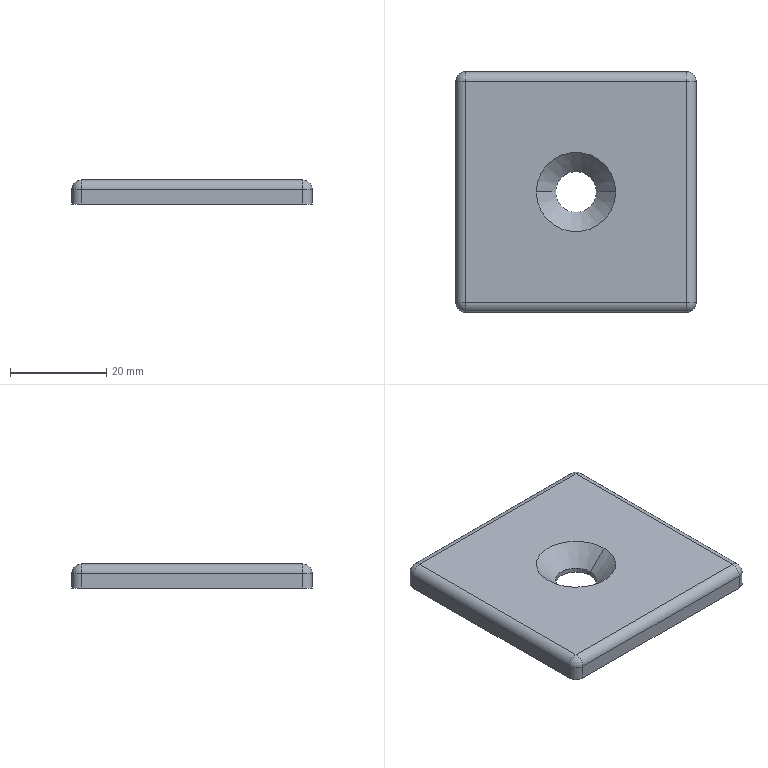Part | NX | features BREP 1 | 1 solid | 22 faces | box 50 x 50 x 5 mm | volume 11752 mm3 | cylinder 10 | plane 6 | sphere 4 | cone 2 | commonest cylinder face diameters 4 x8 8.5 x2
STEP:
#1=CARTESIAN_POINT('',(-4.25,0.,1.));
#2=VERTEX_POINT('',#1);
#3=CARTESIAN_POINT('',(4.25,0.,1.));
#4=VERTEX_POINT('',#3);
#5=CARTESIAN_POINT('',(0.,0.,1.));
#6=DIRECTION('',(0.,0.,1.));
#7=DIRECTION('',(-1.,0.,0.));
#8=AXIS2_PLACEMENT_3D('',#5,#6,#7);
#9=CIRCLE('',#8,4.25);
#10=EDGE_CURVE('',#2,#4,#9,.T.);
#11=ORIENTED_EDGE('',*,*,#10,.F.);
#12=CARTESIAN_POINT('',(-8.25,0.,5.));
#13=VERTEX_POINT('',#12);
#14=CARTESIAN_POINT('',(-4.25,0.,1.));
#15=DIRECTION('',(-0.7071,0.,0.7071));
#16=VECTOR('',#15,1000.);
#17=LINE('',#14,#16);
#18=EDGE_CURVE('',#13,#2,#17,.F.);
#19=ORIENTED_EDGE('',*,*,#18,.F.);
#20=CARTESIAN_POINT('',(8.25,0.,5.));
#21=VERTEX_POINT('',#20);
#22=CARTESIAN_POINT('',(0.,0.,5.));
#23=DIRECTION('',(0.,0.,-1.));
#24=DIRECTION('',(-1.,0.,0.));
#25=AXIS2_PLACEMENT_3D('',#22,#23,#24);
#26=CIRCLE('',#25,8.25);
#27=EDGE_CURVE('',#21,#13,#26,.T.);
#28=ORIENTED_EDGE('',*,*,#27,.F.);
#29=CARTESIAN_POINT('',(4.25,0.,1.));
#30=DIRECTION('',(0.7071,0.,0.7071));
#31=VECTOR('',#30,1000.);
#32=LINE('',#29,#31);
#33=EDGE_CURVE('',#21,#4,#32,.F.);
#34=ORIENTED_EDGE('',*,*,#33,.T.);
#35=EDGE_LOOP('',(#11,#19,#28,#34));
#36=FACE_BOUND('',#35,.T.);
#37=CARTESIAN_POINT('',(0.,0.,1.));
#38=DIRECTION('',(0.,0.,1.));
#39=DIRECTION('',(1.,0.,0.));
#40=AXIS2_PLACEMENT_3D('',#37,#38,#39);
#41=CONICAL_SURFACE('',#40,4.25,0.7854);
#42=ADVANCED_FACE('',(#36),#41,.F.);
#43=CARTESIAN_POINT('',(-4.25,0.,0.));
#44=VERTEX_POINT('',#43);
#45=CARTESIAN_POINT('',(4.25,0.,0.));
#46=VERTEX_POINT('',#45);
#47=CARTESIAN_POINT('',(0.,0.,0.));
#48=DIRECTION('',(0.,0.,1.));
#49=DIRECTION('',(1.,0.,0.));
#50=AXIS2_PLACEMENT_3D('',#47,#48,#49);
#51=CIRCLE('',#50,4.25);
#52=EDGE_CURVE('',#44,#46,#51,.T.);
#53=ORIENTED_EDGE('',*,*,#52,.F.);
#54=CARTESIAN_POINT('',(-4.25,0.,0.));
#55=DIRECTION('',(0.,0.,1.));
#56=VECTOR('',#55,1000.);
#57=LINE('',#54,#56);
#58=EDGE_CURVE('',#2,#44,#57,.F.);
#59=ORIENTED_EDGE('',*,*,#58,.F.);
#60=ORIENTED_EDGE('',*,*,#10,.T.);
#61=CARTESIAN_POINT('',(4.25,0.,0.));
#62=DIRECTION('',(0.,0.,1.));
#63=VECTOR('',#62,1000.);
#64=LINE('',#61,#63);
#65=EDGE_CURVE('',#4,#46,#64,.F.);
#66=ORIENTED_EDGE('',*,*,#65,.T.);
#67=EDGE_LOOP('',(#53,#59,#60,#66));
#68=FACE_BOUND('',#67,.T.);
#69=CARTESIAN_POINT('',(0.,0.,0.));
#70=DIRECTION('',(0.,0.,1.));
#71=DIRECTION('',(1.,0.,0.));
#72=AXIS2_PLACEMENT_3D('',#69,#70,#71);
#73=CYLINDRICAL_SURFACE('',#72,4.25);
#74=ADVANCED_FACE('',(#68),#73,.F.);
#75=CARTESIAN_POINT('',(25.,-23.,0.));
#76=VERTEX_POINT('',#75);
#77=CARTESIAN_POINT('',(25.,23.,0.));
#78=VERTEX_POINT('',#77);
#79=CARTESIAN_POINT('',(25.,-25.,0.));
#80=DIRECTION('',(0.,1.,0.));
#81=VECTOR('',#80,1000.);
#82=LINE('',#79,#81);
#83=EDGE_CURVE('',#76,#78,#82,.T.);
#84=ORIENTED_EDGE('',*,*,#83,.T.);
#85=CARTESIAN_POINT('',(25.,23.,3.));
#86=VERTEX_POINT('',#85);
#87=CARTESIAN_POINT('',(25.,23.,5.));
#88=DIRECTION('',(0.,0.,1.));
#89=VECTOR('',#88,1000.);
#90=LINE('',#87,#89);
#91=EDGE_CURVE('',#78,#86,#90,.T.);
#92=ORIENTED_EDGE('',*,*,#91,.T.);
#93=CARTESIAN_POINT('',(25.,-23.,3.));
#94=VERTEX_POINT('',#93);
#95=CARTESIAN_POINT('',(25.,-25.,3.));
#96=DIRECTION('',(0.,-1.,0.));
#97=VECTOR('',#96,1000.);
#98=LINE('',#95,#97);
#99=EDGE_CURVE('',#86,#94,#98,.T.);
#100=ORIENTED_EDGE('',*,*,#99,.T.);
#101=CARTESIAN_POINT('',(25.,-23.,5.));
#102=DIRECTION('',(0.,0.,-1.));
#103=VECTOR('',#102,1000.);
#104=LINE('',#101,#103);
#105=EDGE_CURVE('',#94,#76,#104,.T.);
#106=ORIENTED_EDGE('',*,*,#105,.T.);
#107=EDGE_LOOP('',(#84,#92,#100,#106));
#108=FACE_BOUND('',#107,.T.);
#109=CARTESIAN_POINT('',(25.,-25.,5.));
#110=DIRECTION('',(-1.,0.,0.));
#111=DIRECTION('',(0.,0.,1.));
#112=AXIS2_PLACEMENT_3D('',#109,#110,#111);
#113=PLANE('',#112);
#114=ADVANCED_FACE('',(#108),#113,.F.);
#115=CARTESIAN_POINT('',(23.,25.,0.));
#116=VERTEX_POINT('',#115);
#117=CARTESIAN_POINT('',(-23.,25.,0.));
#118=VERTEX_POINT('',#117);
#119=CARTESIAN_POINT('',(-25.,25.,0.));
#120=DIRECTION('',(-1.,0.,0.));
#121=VECTOR('',#120,1000.);
#122=LINE('',#119,#121);
#123=EDGE_CURVE('',#116,#118,#122,.T.);
#124=ORIENTED_EDGE('',*,*,#123,.T.);
#125=CARTESIAN_POINT('',(-23.,25.,3.));
#126=VERTEX_POINT('',#125);
#127=CARTESIAN_POINT('',(-23.,25.,5.));
#128=DIRECTION('',(0.,0.,1.));
#129=VECTOR('',#128,1000.);
#130=LINE('',#127,#129);
#131=EDGE_CURVE('',#118,#126,#130,.T.);
#132=ORIENTED_EDGE('',*,*,#131,.T.);
#133=CARTESIAN_POINT('',(23.,25.,3.));
#134=VERTEX_POINT('',#133);
#135=CARTESIAN_POINT('',(-25.,25.,3.));
#136=DIRECTION('',(1.,0.,0.));
#137=VECTOR('',#136,1000.);
#138=LINE('',#135,#137);
#139=EDGE_CURVE('',#126,#134,#138,.T.);
#140=ORIENTED_EDGE('',*,*,#139,.T.);
#141=CARTESIAN_POINT('',(23.,25.,5.));
#142=DIRECTION('',(0.,0.,-1.));
#143=VECTOR('',#142,1000.);
#144=LINE('',#141,#143);
#145=EDGE_CURVE('',#134,#116,#144,.T.);
#146=ORIENTED_EDGE('',*,*,#145,.T.);
#147=EDGE_LOOP('',(#124,#132,#140,#146));
#148=FACE_BOUND('',#147,.T.);
#149=CARTESIAN_POINT('',(-25.,25.,5.));
#150=DIRECTION('',(0.,-1.,0.));
#151=DIRECTION('',(0.,0.,-1.));
#152=AXIS2_PLACEMENT_3D('',#149,#150,#151);
#153=PLANE('',#152);
#154=ADVANCED_FACE('',(#148),#153,.F.);
#155=CARTESIAN_POINT('',(-25.,-23.,3.));
#156=VERTEX_POINT('',#155);
#157=CARTESIAN_POINT('',(-25.,23.,3.));
#158=VERTEX_POINT('',#157);
#159=CARTESIAN_POINT('',(-25.,-25.,3.));
#160=DIRECTION('',(0.,1.,0.));
#161=VECTOR('',#160,1000.);
#162=LINE('',#159,#161);
#163=EDGE_CURVE('',#156,#158,#162,.T.);
#164=ORIENTED_EDGE('',*,*,#163,.T.);
#165=CARTESIAN_POINT('',(-25.,23.,0.));
#166=VERTEX_POINT('',#165);
#167=CARTESIAN_POINT('',(-25.,23.,5.));
#168=DIRECTION('',(0.,0.,-1.));
#169=VECTOR('',#168,1000.);
#170=LINE('',#167,#169);
#171=EDGE_CURVE('',#158,#166,#170,.T.);
#172=ORIENTED_EDGE('',*,*,#171,.T.);
#173=CARTESIAN_POINT('',(-25.,-23.,0.));
#174=VERTEX_POINT('',#173);
#175=CARTESIAN_POINT('',(-25.,-25.,0.));
#176=DIRECTION('',(0.,-1.,0.));
#177=VECTOR('',#176,1000.);
#178=LINE('',#175,#177);
#179=EDGE_CURVE('',#166,#174,#178,.T.);
#180=ORIENTED_EDGE('',*,*,#179,.T.);
#181=CARTESIAN_POINT('',(-25.,-23.,5.));
#182=DIRECTION('',(0.,0.,1.));
#183=VECTOR('',#182,1000.);
#184=LINE('',#181,#183);
#185=EDGE_CURVE('',#174,#156,#184,.T.);
#186=ORIENTED_EDGE('',*,*,#185,.T.);
#187=EDGE_LOOP('',(#164,#172,#180,#186));
#188=FACE_BOUND('',#187,.T.);
#189=CARTESIAN_POINT('',(-25.,-25.,5.));
#190=DIRECTION('',(1.,0.,0.));
#191=DIRECTION('',(0.,1.,0.));
#192=AXIS2_PLACEMENT_3D('',#189,#190,#191);
#193=PLANE('',#192);
#194=ADVANCED_FACE('',(#188),#193,.F.);
#195=CARTESIAN_POINT('',(-23.,-25.,0.));
#196=VERTEX_POINT('',#195);
#197=CARTESIAN_POINT('',(23.,-25.,0.));
#198=VERTEX_POINT('',#197);
#199=CARTESIAN_POINT('',(-25.,-25.,0.));
#200=DIRECTION('',(1.,0.,0.));
#201=VECTOR('',#200,1000.);
#202=LINE('',#199,#201);
#203=EDGE_CURVE('',#196,#198,#202,.T.);
#204=ORIENTED_EDGE('',*,*,#203,.T.);
#205=CARTESIAN_POINT('',(23.,-25.,3.));
#206=VERTEX_POINT('',#205);
#207=CARTESIAN_POINT('',(23.,-25.,5.));
#208=DIRECTION('',(0.,0.,1.));
#209=VECTOR('',#208,1000.);
#210=LINE('',#207,#209);
#211=EDGE_CURVE('',#198,#206,#210,.T.);
#212=ORIENTED_EDGE('',*,*,#211,.T.);
#213=CARTESIAN_POINT('',(-23.,-25.,3.));
#214=VERTEX_POINT('',#213);
#215=CARTESIAN_POINT('',(-25.,-25.,3.));
#216=DIRECTION('',(-1.,0.,0.));
#217=VECTOR('',#216,1000.);
#218=LINE('',#215,#217);
#219=EDGE_CURVE('',#206,#214,#218,.T.);
#220=ORIENTED_EDGE('',*,*,#219,.T.);
#221=CARTESIAN_POINT('',(-23.,-25.,5.));
#222=DIRECTION('',(0.,0.,-1.));
#223=VECTOR('',#222,1000.);
#224=LINE('',#221,#223);
#225=EDGE_CURVE('',#214,#196,#224,.T.);
#226=ORIENTED_EDGE('',*,*,#225,.T.);
#227=EDGE_LOOP('',(#204,#212,#220,#226));
#228=FACE_BOUND('',#227,.T.);
#229=CARTESIAN_POINT('',(-25.,-25.,5.));
#230=DIRECTION('',(0.,1.,0.));
#231=DIRECTION('',(1.,0.,0.));
#232=AXIS2_PLACEMENT_3D('',#229,#230,#231);
#233=PLANE('',#232);
#234=ADVANCED_FACE('',(#228),#233,.F.);
#235=CARTESIAN_POINT('',(-23.,23.,5.));
#236=VERTEX_POINT('',#235);
#237=CARTESIAN_POINT('',(-23.,-23.,5.));
#238=VERTEX_POINT('',#237);
#239=CARTESIAN_POINT('',(-23.,0.,5.));
#240=DIRECTION('',(0.,-1.,0.));
#241=VECTOR('',#240,1000.);
#242=LINE('',#239,#241);
#243=EDGE_CURVE('',#236,#238,#242,.T.);
#244=ORIENTED_EDGE('',*,*,#243,.T.);
#245=CARTESIAN_POINT('',(23.,-23.,5.));
#246=VERTEX_POINT('',#245);
#247=CARTESIAN_POINT('',(0.,-23.,5.));
#248=DIRECTION('',(1.,0.,0.));
#249=VECTOR('',#248,1000.);
#250=LINE('',#247,#249);
#251=EDGE_CURVE('',#238,#246,#250,.T.);
#252=ORIENTED_EDGE('',*,*,#251,.T.);
#253=CARTESIAN_POINT('',(23.,23.,5.));
#254=VERTEX_POINT('',#253);
#255=CARTESIAN_POINT('',(23.,0.,5.));
#256=DIRECTION('',(0.,1.,0.));
#257=VECTOR('',#256,1000.);
#258=LINE('',#255,#257);
#259=EDGE_CURVE('',#246,#254,#258,.T.);
#260=ORIENTED_EDGE('',*,*,#259,.T.);
#261=CARTESIAN_POINT('',(0.,23.,5.));
#262=DIRECTION('',(-1.,0.,0.));
#263=VECTOR('',#262,1000.);
#264=LINE('',#261,#263);
#265=EDGE_CURVE('',#254,#236,#264,.T.);
#266=ORIENTED_EDGE('',*,*,#265,.T.);
#267=EDGE_LOOP('',(#244,#252,#260,#266));
#268=FACE_BOUND('',#267,.T.);
#269=ORIENTED_EDGE('',*,*,#27,.T.);
#270=CARTESIAN_POINT('',(0.,0.,5.));
#271=DIRECTION('',(0.,0.,-1.));
#272=DIRECTION('',(-1.,0.,0.));
#273=AXIS2_PLACEMENT_3D('',#270,#271,#272);
#274=CIRCLE('',#273,8.25);
#275=EDGE_CURVE('',#13,#21,#274,.T.);
#276=ORIENTED_EDGE('',*,*,#275,.T.);
#277=EDGE_LOOP('',(#269,#276));
#278=FACE_BOUND('',#277,.T.);
#279=CARTESIAN_POINT('',(0.,0.,5.));
#280=DIRECTION('',(0.,0.,-1.));
#281=DIRECTION('',(0.,-1.,0.));
#282=AXIS2_PLACEMENT_3D('',#279,#280,#281);
#283=PLANE('',#282);
#284=ADVANCED_FACE('',(#268,#278),#283,.F.);
#285=ORIENTED_EDGE('',*,*,#179,.F.);
#286=CARTESIAN_POINT('',(-23.,23.,0.));
#287=DIRECTION('',(0.,0.,-1.));
#288=DIRECTION('',(-1.,0.,0.));
#289=AXIS2_PLACEMENT_3D('',#286,#287,#288);
#290=CIRCLE('',#289,2.);
#291=EDGE_CURVE('',#166,#118,#290,.T.);
#292=ORIENTED_EDGE('',*,*,#291,.T.);
#293=ORIENTED_EDGE('',*,*,#123,.F.);
#294=CARTESIAN_POINT('',(23.,23.,0.));
#295=DIRECTION('',(0.,0.,-1.));
#296=DIRECTION('',(-1.,0.,0.));
#297=AXIS2_PLACEMENT_3D('',#294,#295,#296);
#298=CIRCLE('',#297,2.);
#299=EDGE_CURVE('',#116,#78,#298,.T.);
#300=ORIENTED_EDGE('',*,*,#299,.T.);
#301=ORIENTED_EDGE('',*,*,#83,.F.);
#302=CARTESIAN_POINT('',(23.,-23.,0.));
#303=DIRECTION('',(0.,0.,-1.));
#304=DIRECTION('',(-1.,0.,0.));
#305=AXIS2_PLACEMENT_3D('',#302,#303,#304);
#306=CIRCLE('',#305,2.);
#307=EDGE_CURVE('',#76,#198,#306,.T.);
#308=ORIENTED_EDGE('',*,*,#307,.T.);
#309=ORIENTED_EDGE('',*,*,#203,.F.);
#310=CARTESIAN_POINT('',(-23.,-23.,0.));
#311=DIRECTION('',(0.,0.,-1.));
#312=DIRECTION('',(-1.,0.,0.));
#313=AXIS2_PLACEMENT_3D('',#310,#311,#312);
#314=CIRCLE('',#313,2.);
#315=EDGE_CURVE('',#196,#174,#314,.T.);
#316=ORIENTED_EDGE('',*,*,#315,.T.);
#317=EDGE_LOOP('',(#285,#292,#293,#300,#301,#308,#309,#316));
#318=FACE_BOUND('',#317,.T.);
#319=CARTESIAN_POINT('',(0.,0.,0.));
#320=DIRECTION('',(0.,0.,1.));
#321=DIRECTION('',(1.,0.,0.));
#322=AXIS2_PLACEMENT_3D('',#319,#320,#321);
#323=CIRCLE('',#322,4.25);
#324=EDGE_CURVE('',#46,#44,#323,.T.);
#325=ORIENTED_EDGE('',*,*,#324,.T.);
#326=ORIENTED_EDGE('',*,*,#52,.T.);
#327=EDGE_LOOP('',(#325,#326));
#328=FACE_BOUND('',#327,.T.);
#329=CARTESIAN_POINT('',(0.,0.,0.));
#330=DIRECTION('',(0.,0.,-1.));
#331=DIRECTION('',(0.,-1.,0.));
#332=AXIS2_PLACEMENT_3D('',#329,#330,#331);
#333=PLANE('',#332);
#334=ADVANCED_FACE('',(#318,#328),#333,.T.);
#335=ORIENTED_EDGE('',*,*,#291,.F.);
#336=ORIENTED_EDGE('',*,*,#171,.F.);
#337=CARTESIAN_POINT('',(-23.,23.,3.));
#338=DIRECTION('',(0.,0.,1.));
#339=DIRECTION('',(1.,0.,0.));
#340=AXIS2_PLACEMENT_3D('',#337,#338,#339);
#341=CIRCLE('',#340,2.);
#342=EDGE_CURVE('',#126,#158,#341,.T.);
#343=ORIENTED_EDGE('',*,*,#342,.F.);
#344=ORIENTED_EDGE('',*,*,#131,.F.);
#345=EDGE_LOOP('',(#335,#336,#343,#344));
#346=FACE_BOUND('',#345,.T.);
#347=CARTESIAN_POINT('',(-23.,23.,5.));
#348=DIRECTION('',(0.,0.,-1.));
#349=DIRECTION('',(-1.,0.,0.));
#350=AXIS2_PLACEMENT_3D('',#347,#348,#349);
#351=CYLINDRICAL_SURFACE('',#350,2.);
#352=ADVANCED_FACE('',(#346),#351,.T.);
#353=CARTESIAN_POINT('',(23.,23.,3.));
#354=DIRECTION('',(1.,0.,0.));
#355=DIRECTION('',(0.,0.,-1.));
#356=AXIS2_PLACEMENT_3D('',#353,#354,#355);
#357=CIRCLE('',#356,2.);
#358=EDGE_CURVE('',#134,#254,#357,.T.);
#359=ORIENTED_EDGE('',*,*,#358,.F.);
#360=ORIENTED_EDGE('',*,*,#139,.F.);
#361=CARTESIAN_POINT('',(-23.,23.,3.));
#362=DIRECTION('',(-1.,0.,0.));
#363=DIRECTION('',(0.,0.,1.));
#364=AXIS2_PLACEMENT_3D('',#361,#362,#363);
#365=CIRCLE('',#364,2.);
#366=EDGE_CURVE('',#236,#126,#365,.T.);
#367=ORIENTED_EDGE('',*,*,#366,.F.);
#368=ORIENTED_EDGE('',*,*,#265,.F.);
#369=EDGE_LOOP('',(#359,#360,#367,#368));
#370=FACE_BOUND('',#369,.T.);
#371=CARTESIAN_POINT('',(0.,23.,3.));
#372=DIRECTION('',(-1.,0.,0.));
#373=DIRECTION('',(0.,0.,1.));
#374=AXIS2_PLACEMENT_3D('',#371,#372,#373);
#375=CYLINDRICAL_SURFACE('',#374,2.);
#376=ADVANCED_FACE('',(#370),#375,.T.);
#377=ORIENTED_EDGE('',*,*,#299,.F.);
#378=ORIENTED_EDGE('',*,*,#145,.F.);
#379=CARTESIAN_POINT('',(23.,23.,3.));
#380=DIRECTION('',(0.,0.,1.));
#381=DIRECTION('',(1.,0.,0.));
#382=AXIS2_PLACEMENT_3D('',#379,#380,#381);
#383=CIRCLE('',#382,2.);
#384=EDGE_CURVE('',#86,#134,#383,.T.);
#385=ORIENTED_EDGE('',*,*,#384,.F.);
#386=ORIENTED_EDGE('',*,*,#91,.F.);
#387=EDGE_LOOP('',(#377,#378,#385,#386));
#388=FACE_BOUND('',#387,.T.);
#389=CARTESIAN_POINT('',(23.,23.,5.));
#390=DIRECTION('',(0.,0.,-1.));
#391=DIRECTION('',(-1.,0.,0.));
#392=AXIS2_PLACEMENT_3D('',#389,#390,#391);
#393=CYLINDRICAL_SURFACE('',#392,2.);
#394=ADVANCED_FACE('',(#388),#393,.T.);
#395=ORIENTED_EDGE('',*,*,#366,.T.);
#396=ORIENTED_EDGE('',*,*,#342,.T.);
#397=CARTESIAN_POINT('',(-23.,23.,3.));
#398=DIRECTION('',(0.,-1.,0.));
#399=DIRECTION('',(0.,0.,1.));
#400=AXIS2_PLACEMENT_3D('',#397,#398,#399);
#401=CIRCLE('',#400,2.);
#402=EDGE_CURVE('',#236,#158,#401,.T.);
#403=ORIENTED_EDGE('',*,*,#402,.F.);
#404=EDGE_LOOP('',(#395,#396,#403));
#405=FACE_BOUND('',#404,.T.);
#406=CARTESIAN_POINT('',(-23.,23.,3.));
#407=DIRECTION('',(0.,0.,-1.));
#408=DIRECTION('',(1.,0.,0.));
#409=AXIS2_PLACEMENT_3D('',#406,#407,#408);
#410=SPHERICAL_SURFACE('',#409,2.);
#411=ADVANCED_FACE('',(#405),#410,.T.);
#412=ORIENTED_EDGE('',*,*,#384,.T.);
#413=ORIENTED_EDGE('',*,*,#358,.T.);
#414=CARTESIAN_POINT('',(23.,23.,3.));
#415=DIRECTION('',(0.,-1.,0.));
#416=DIRECTION('',(0.,0.,1.));
#417=AXIS2_PLACEMENT_3D('',#414,#415,#416);
#418=CIRCLE('',#417,2.);
#419=EDGE_CURVE('',#86,#254,#418,.T.);
#420=ORIENTED_EDGE('',*,*,#419,.F.);
#421=EDGE_LOOP('',(#412,#413,#420));
#422=FACE_BOUND('',#421,.T.);
#423=CARTESIAN_POINT('',(23.,23.,3.));
#424=DIRECTION('',(0.,0.,-1.));
#425=DIRECTION('',(1.,0.,0.));
#426=AXIS2_PLACEMENT_3D('',#423,#424,#425);
#427=SPHERICAL_SURFACE('',#426,2.);
#428=ADVANCED_FACE('',(#422),#427,.T.);
#429=ORIENTED_EDGE('',*,*,#315,.F.);
#430=ORIENTED_EDGE('',*,*,#225,.F.);
#431=CARTESIAN_POINT('',(-23.,-23.,3.));
#432=DIRECTION('',(0.,0.,1.));
#433=DIRECTION('',(1.,0.,0.));
#434=AXIS2_PLACEMENT_3D('',#431,#432,#433);
#435=CIRCLE('',#434,2.);
#436=EDGE_CURVE('',#156,#214,#435,.T.);
#437=ORIENTED_EDGE('',*,*,#436,.F.);
#438=ORIENTED_EDGE('',*,*,#185,.F.);
#439=EDGE_LOOP('',(#429,#430,#437,#438));
#440=FACE_BOUND('',#439,.T.);
#441=CARTESIAN_POINT('',(-23.,-23.,5.));
#442=DIRECTION('',(0.,0.,-1.));
#443=DIRECTION('',(-1.,0.,0.));
#444=AXIS2_PLACEMENT_3D('',#441,#442,#443);
#445=CYLINDRICAL_SURFACE('',#444,2.);
#446=ADVANCED_FACE('',(#440),#445,.T.);
#447=ORIENTED_EDGE('',*,*,#402,.T.);
#448=ORIENTED_EDGE('',*,*,#163,.F.);
#449=CARTESIAN_POINT('',(-23.,-23.,3.));
#450=DIRECTION('',(0.,-1.,0.));
#451=DIRECTION('',(0.,0.,-1.));
#452=AXIS2_PLACEMENT_3D('',#449,#450,#451);
#453=CIRCLE('',#452,2.);
#454=EDGE_CURVE('',#238,#156,#453,.T.);
#455=ORIENTED_EDGE('',*,*,#454,.F.);
#456=ORIENTED_EDGE('',*,*,#243,.F.);
#457=EDGE_LOOP('',(#447,#448,#455,#456));
#458=FACE_BOUND('',#457,.T.);
#459=CARTESIAN_POINT('',(-23.,0.,3.));
#460=DIRECTION('',(0.,-1.,0.));
#461=DIRECTION('',(0.,0.,-1.));
#462=AXIS2_PLACEMENT_3D('',#459,#460,#461);
#463=CYLINDRICAL_SURFACE('',#462,2.);
#464=ADVANCED_FACE('',(#458),#463,.T.);
#465=ORIENTED_EDGE('',*,*,#419,.T.);
#466=ORIENTED_EDGE('',*,*,#259,.F.);
#467=CARTESIAN_POINT('',(23.,-23.,3.));
#468=DIRECTION('',(0.,-1.,0.));
#469=DIRECTION('',(0.,0.,-1.));
#470=AXIS2_PLACEMENT_3D('',#467,#468,#469);
#471=CIRCLE('',#470,2.);
#472=EDGE_CURVE('',#94,#246,#471,.T.);
#473=ORIENTED_EDGE('',*,*,#472,.F.);
#474=ORIENTED_EDGE('',*,*,#99,.F.);
#475=EDGE_LOOP('',(#465,#466,#473,#474));
#476=FACE_BOUND('',#475,.T.);
#477=CARTESIAN_POINT('',(23.,0.,3.));
#478=DIRECTION('',(0.,1.,0.));
#479=DIRECTION('',(0.,0.,1.));
#480=AXIS2_PLACEMENT_3D('',#477,#478,#479);
#481=CYLINDRICAL_SURFACE('',#480,2.);
#482=ADVANCED_FACE('',(#476),#481,.T.);
#483=ORIENTED_EDGE('',*,*,#307,.F.);
#484=ORIENTED_EDGE('',*,*,#105,.F.);
#485=CARTESIAN_POINT('',(23.,-23.,3.));
#486=DIRECTION('',(0.,0.,1.));
#487=DIRECTION('',(1.,0.,0.));
#488=AXIS2_PLACEMENT_3D('',#485,#486,#487);
#489=CIRCLE('',#488,2.);
#490=EDGE_CURVE('',#206,#94,#489,.T.);
#491=ORIENTED_EDGE('',*,*,#490,.F.);
#492=ORIENTED_EDGE('',*,*,#211,.F.);
#493=EDGE_LOOP('',(#483,#484,#491,#492));
#494=FACE_BOUND('',#493,.T.);
#495=CARTESIAN_POINT('',(23.,-23.,5.));
#496=DIRECTION('',(0.,0.,-1.));
#497=DIRECTION('',(-1.,0.,0.));
#498=AXIS2_PLACEMENT_3D('',#495,#496,#497);
#499=CYLINDRICAL_SURFACE('',#498,2.);
#500=ADVANCED_FACE('',(#494),#499,.T.);
#501=ORIENTED_EDGE('',*,*,#454,.T.);
#502=ORIENTED_EDGE('',*,*,#436,.T.);
#503=CARTESIAN_POINT('',(-23.,-23.,3.));
#504=DIRECTION('',(1.,0.,0.));
#505=DIRECTION('',(0.,0.,1.));
#506=AXIS2_PLACEMENT_3D('',#503,#504,#505);
#507=CIRCLE('',#506,2.);
#508=EDGE_CURVE('',#238,#214,#507,.T.);
#509=ORIENTED_EDGE('',*,*,#508,.F.);
#510=EDGE_LOOP('',(#501,#502,#509));
#511=FACE_BOUND('',#510,.T.);
#512=CARTESIAN_POINT('',(-23.,-23.,3.));
#513=DIRECTION('',(0.,0.,-1.));
#514=DIRECTION('',(1.,0.,0.));
#515=AXIS2_PLACEMENT_3D('',#512,#513,#514);
#516=SPHERICAL_SURFACE('',#515,2.);
#517=ADVANCED_FACE('',(#511),#516,.T.);
#518=ORIENTED_EDGE('',*,*,#490,.T.);
#519=ORIENTED_EDGE('',*,*,#472,.T.);
#520=CARTESIAN_POINT('',(23.,-23.,3.));
#521=DIRECTION('',(-1.,0.,0.));
#522=DIRECTION('',(0.,0.,-1.));
#523=AXIS2_PLACEMENT_3D('',#520,#521,#522);
#524=CIRCLE('',#523,2.);
#525=EDGE_CURVE('',#206,#246,#524,.T.);
#526=ORIENTED_EDGE('',*,*,#525,.F.);
#527=EDGE_LOOP('',(#518,#519,#526));
#528=FACE_BOUND('',#527,.T.);
#529=CARTESIAN_POINT('',(23.,-23.,3.));
#530=DIRECTION('',(0.,0.,-1.));
#531=DIRECTION('',(1.,0.,0.));
#532=AXIS2_PLACEMENT_3D('',#529,#530,#531);
#533=SPHERICAL_SURFACE('',#532,2.);
#534=ADVANCED_FACE('',(#528),#533,.T.);
#535=ORIENTED_EDGE('',*,*,#508,.T.);
#536=ORIENTED_EDGE('',*,*,#219,.F.);
#537=ORIENTED_EDGE('',*,*,#525,.T.);
#538=ORIENTED_EDGE('',*,*,#251,.F.);
#539=EDGE_LOOP('',(#535,#536,#537,#538));
#540=FACE_BOUND('',#539,.T.);
#541=CARTESIAN_POINT('',(0.,-23.,3.));
#542=DIRECTION('',(1.,0.,0.));
#543=DIRECTION('',(0.,0.,-1.));
#544=AXIS2_PLACEMENT_3D('',#541,#542,#543);
#545=CYLINDRICAL_SURFACE('',#544,2.);
#546=ADVANCED_FACE('',(#540),#545,.T.);
#547=ORIENTED_EDGE('',*,*,#58,.T.);
#548=ORIENTED_EDGE('',*,*,#324,.F.);
#549=ORIENTED_EDGE('',*,*,#65,.F.);
#550=CARTESIAN_POINT('',(0.,0.,1.));
#551=DIRECTION('',(0.,0.,1.));
#552=DIRECTION('',(-1.,0.,0.));
#553=AXIS2_PLACEMENT_3D('',#550,#551,#552);
#554=CIRCLE('',#553,4.25);
#555=EDGE_CURVE('',#4,#2,#554,.T.);
#556=ORIENTED_EDGE('',*,*,#555,.T.);
#557=EDGE_LOOP('',(#547,#548,#549,#556));
#558=FACE_BOUND('',#557,.T.);
#559=CARTESIAN_POINT('',(0.,0.,0.));
#560=DIRECTION('',(0.,0.,1.));
#561=DIRECTION('',(1.,0.,0.));
#562=AXIS2_PLACEMENT_3D('',#559,#560,#561);
#563=CYLINDRICAL_SURFACE('',#562,4.25);
#564=ADVANCED_FACE('',(#558),#563,.F.);
#565=ORIENTED_EDGE('',*,*,#18,.T.);
#566=ORIENTED_EDGE('',*,*,#555,.F.);
#567=ORIENTED_EDGE('',*,*,#33,.F.);
#568=ORIENTED_EDGE('',*,*,#275,.F.);
#569=EDGE_LOOP('',(#565,#566,#567,#568));
#570=FACE_BOUND('',#569,.T.);
#571=CARTESIAN_POINT('',(0.,0.,1.));
#572=DIRECTION('',(0.,0.,1.));
#573=DIRECTION('',(1.,0.,0.));
#574=AXIS2_PLACEMENT_3D('',#571,#572,#573);
#575=CONICAL_SURFACE('',#574,4.25,0.7854);
#576=ADVANCED_FACE('',(#570),#575,.F.);
#577=CLOSED_SHELL('',(#42,#74,#114,#154,#194,#234,#284,#334,#352,#376,#394,#411,#428,#446,#464,#482,#500,#517,#534,#546,#564,#576));
#578=MANIFOLD_SOLID_BREP('',#577);
#579=(LENGTH_UNIT()NAMED_UNIT(*)SI_UNIT(.MILLI.,.METRE.));
#580=UNCERTAINTY_MEASURE_WITH_UNIT(LENGTH_MEASURE(0.00001),#579,'','');
#581=(NAMED_UNIT(*)PLANE_ANGLE_UNIT()SI_UNIT($,.RADIAN.));
#582=(NAMED_UNIT(*)SI_UNIT($,.STERADIAN.)SOLID_ANGLE_UNIT());
#583=(GEOMETRIC_REPRESENTATION_CONTEXT(3)GLOBAL_UNCERTAINTY_ASSIGNED_CONTEXT((#580))GLOBAL_UNIT_ASSIGNED_CONTEXT((#579,#581,#582))REPRESENTATION_CONTEXT('',''));
#584=ADVANCED_BREP_SHAPE_REPRESENTATION('',(#578),#583);